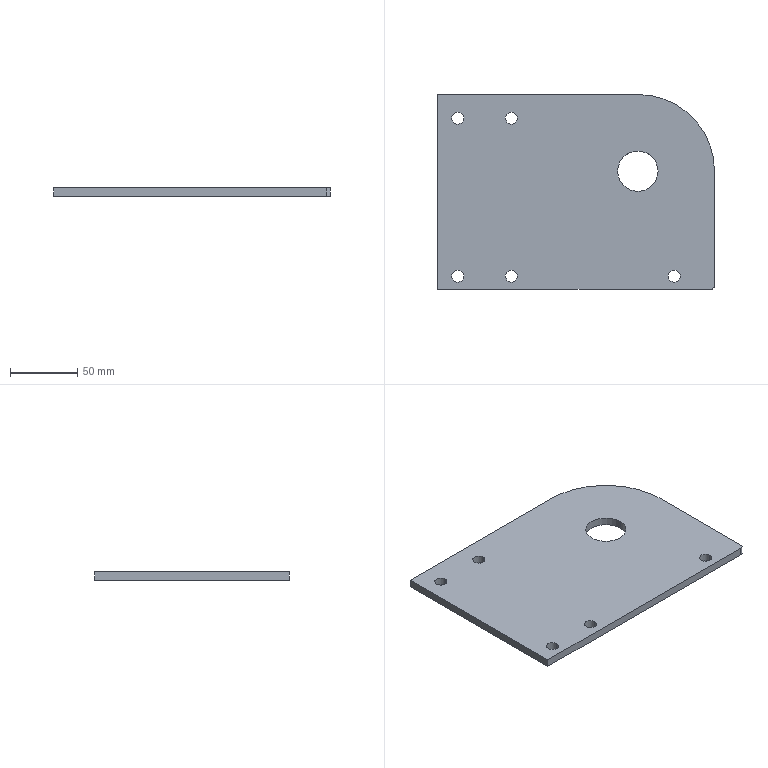Part | SolidWorks | features ICE 6, Fillet 5, HoleWzd 2, CirPattern 1, Extrusion 1 | 1 solid | 20 faces | box 206 x 145 x 6 mm | volume 168875 mm3 | cylinder 14 | plane 6 | commonest cylinder face diameters 9 x10 30 x2 6 x1 114 x1
STEP:
#1=CARTESIAN_POINT('',(68.5,-62.5,0.));
#2=VERTEX_POINT('',#1);
#3=CARTESIAN_POINT('',(77.5,-62.5,0.));
#4=VERTEX_POINT('',#3);
#5=CARTESIAN_POINT('',(73.,-62.5,0.));
#6=DIRECTION('',(0.,0.,1.));
#7=DIRECTION('',(1.,0.,0.));
#8=AXIS2_PLACEMENT_3D('',#5,#6,#7);
#9=CIRCLE('',#8,4.5);
#10=EDGE_CURVE('',#2,#4,#9,.T.);
#11=ORIENTED_EDGE('',*,*,#10,.F.);
#12=CARTESIAN_POINT('',(68.5,-62.5,6.));
#13=VERTEX_POINT('',#12);
#14=CARTESIAN_POINT('',(68.5,-62.5,0.));
#15=DIRECTION('',(0.,0.,1.));
#16=VECTOR('',#15,1000.);
#17=LINE('',#14,#16);
#18=EDGE_CURVE('',#2,#13,#17,.T.);
#19=ORIENTED_EDGE('',*,*,#18,.T.);
#20=CARTESIAN_POINT('',(77.5,-62.5,6.));
#21=VERTEX_POINT('',#20);
#22=CARTESIAN_POINT('',(73.,-62.5,6.));
#23=DIRECTION('',(0.,0.,1.));
#24=DIRECTION('',(1.,0.,0.));
#25=AXIS2_PLACEMENT_3D('',#22,#23,#24);
#26=CIRCLE('',#25,4.5);
#27=EDGE_CURVE('',#13,#21,#26,.T.);
#28=ORIENTED_EDGE('',*,*,#27,.T.);
#29=CARTESIAN_POINT('',(77.5,-62.5,0.));
#30=DIRECTION('',(0.,0.,1.));
#31=VECTOR('',#30,1000.);
#32=LINE('',#29,#31);
#33=EDGE_CURVE('',#4,#21,#32,.T.);
#34=ORIENTED_EDGE('',*,*,#33,.F.);
#35=EDGE_LOOP('',(#11,#19,#28,#34));
#36=FACE_OUTER_BOUND('',#35,.T.);
#37=CARTESIAN_POINT('',(73.,-62.5,0.));
#38=DIRECTION('',(0.,0.,1.));
#39=DIRECTION('',(1.,0.,0.));
#40=AXIS2_PLACEMENT_3D('',#37,#38,#39);
#41=CYLINDRICAL_SURFACE('',#40,4.5);
#42=ADVANCED_FACE('',(#36),#41,.F.);
#43=CARTESIAN_POINT('',(31.,15.5,0.));
#44=VERTEX_POINT('',#43);
#45=CARTESIAN_POINT('',(61.,15.5,0.));
#46=VERTEX_POINT('',#45);
#47=CARTESIAN_POINT('',(46.,15.5,0.));
#48=DIRECTION('',(0.,0.,1.));
#49=DIRECTION('',(1.,0.,0.));
#50=AXIS2_PLACEMENT_3D('',#47,#48,#49);
#51=CIRCLE('',#50,15.);
#52=EDGE_CURVE('',#44,#46,#51,.T.);
#53=ORIENTED_EDGE('',*,*,#52,.F.);
#54=CARTESIAN_POINT('',(31.,15.5,6.));
#55=VERTEX_POINT('',#54);
#56=CARTESIAN_POINT('',(31.,15.5,0.));
#57=DIRECTION('',(0.,0.,1.));
#58=VECTOR('',#57,1000.);
#59=LINE('',#56,#58);
#60=EDGE_CURVE('',#44,#55,#59,.T.);
#61=ORIENTED_EDGE('',*,*,#60,.T.);
#62=CARTESIAN_POINT('',(61.,15.5,6.));
#63=VERTEX_POINT('',#62);
#64=CARTESIAN_POINT('',(46.,15.5,6.));
#65=DIRECTION('',(0.,0.,1.));
#66=DIRECTION('',(1.,0.,0.));
#67=AXIS2_PLACEMENT_3D('',#64,#65,#66);
#68=CIRCLE('',#67,15.);
#69=EDGE_CURVE('',#55,#63,#68,.T.);
#70=ORIENTED_EDGE('',*,*,#69,.T.);
#71=CARTESIAN_POINT('',(61.,15.5,0.));
#72=DIRECTION('',(0.,0.,1.));
#73=VECTOR('',#72,1000.);
#74=LINE('',#71,#73);
#75=EDGE_CURVE('',#46,#63,#74,.T.);
#76=ORIENTED_EDGE('',*,*,#75,.F.);
#77=EDGE_LOOP('',(#53,#61,#70,#76));
#78=FACE_OUTER_BOUND('',#77,.T.);
#79=CARTESIAN_POINT('',(46.,15.5,0.));
#80=DIRECTION('',(0.,0.,1.));
#81=DIRECTION('',(1.,0.,0.));
#82=AXIS2_PLACEMENT_3D('',#79,#80,#81);
#83=CYLINDRICAL_SURFACE('',#82,15.);
#84=ADVANCED_FACE('',(#78),#83,.F.);
#85=CARTESIAN_POINT('',(-52.5,-62.5,0.));
#86=VERTEX_POINT('',#85);
#87=CARTESIAN_POINT('',(-43.5,-62.5,0.));
#88=VERTEX_POINT('',#87);
#89=CARTESIAN_POINT('',(-48.,-62.5,0.));
#90=DIRECTION('',(0.,0.,1.));
#91=DIRECTION('',(1.,0.,0.));
#92=AXIS2_PLACEMENT_3D('',#89,#90,#91);
#93=CIRCLE('',#92,4.5);
#94=EDGE_CURVE('',#86,#88,#93,.T.);
#95=ORIENTED_EDGE('',*,*,#94,.F.);
#96=CARTESIAN_POINT('',(-52.5,-62.5,6.));
#97=VERTEX_POINT('',#96);
#98=CARTESIAN_POINT('',(-52.5,-62.5,0.));
#99=DIRECTION('',(0.,0.,1.));
#100=VECTOR('',#99,1000.);
#101=LINE('',#98,#100);
#102=EDGE_CURVE('',#86,#97,#101,.T.);
#103=ORIENTED_EDGE('',*,*,#102,.T.);
#104=CARTESIAN_POINT('',(-43.5,-62.5,6.));
#105=VERTEX_POINT('',#104);
#106=CARTESIAN_POINT('',(-48.,-62.5,6.));
#107=DIRECTION('',(0.,0.,1.));
#108=DIRECTION('',(1.,0.,0.));
#109=AXIS2_PLACEMENT_3D('',#106,#107,#108);
#110=CIRCLE('',#109,4.5);
#111=EDGE_CURVE('',#97,#105,#110,.T.);
#112=ORIENTED_EDGE('',*,*,#111,.T.);
#113=CARTESIAN_POINT('',(-43.5,-62.5,0.));
#114=DIRECTION('',(0.,0.,1.));
#115=VECTOR('',#114,1000.);
#116=LINE('',#113,#115);
#117=EDGE_CURVE('',#88,#105,#116,.T.);
#118=ORIENTED_EDGE('',*,*,#117,.F.);
#119=EDGE_LOOP('',(#95,#103,#112,#118));
#120=FACE_OUTER_BOUND('',#119,.T.);
#121=CARTESIAN_POINT('',(-48.,-62.5,0.));
#122=DIRECTION('',(0.,0.,1.));
#123=DIRECTION('',(1.,0.,0.));
#124=AXIS2_PLACEMENT_3D('',#121,#122,#123);
#125=CYLINDRICAL_SURFACE('',#124,4.5);
#126=ADVANCED_FACE('',(#120),#125,.F.);
#127=CARTESIAN_POINT('',(-92.5,-62.5,0.));
#128=VERTEX_POINT('',#127);
#129=CARTESIAN_POINT('',(-83.5,-62.5,0.));
#130=VERTEX_POINT('',#129);
#131=CARTESIAN_POINT('',(-88.,-62.5,0.));
#132=DIRECTION('',(0.,0.,1.));
#133=DIRECTION('',(1.,0.,0.));
#134=AXIS2_PLACEMENT_3D('',#131,#132,#133);
#135=CIRCLE('',#134,4.5);
#136=EDGE_CURVE('',#128,#130,#135,.T.);
#137=ORIENTED_EDGE('',*,*,#136,.F.);
#138=CARTESIAN_POINT('',(-92.5,-62.5,6.));
#139=VERTEX_POINT('',#138);
#140=CARTESIAN_POINT('',(-92.5,-62.5,0.));
#141=DIRECTION('',(0.,0.,1.));
#142=VECTOR('',#141,1000.);
#143=LINE('',#140,#142);
#144=EDGE_CURVE('',#128,#139,#143,.T.);
#145=ORIENTED_EDGE('',*,*,#144,.T.);
#146=CARTESIAN_POINT('',(-83.5,-62.5,6.));
#147=VERTEX_POINT('',#146);
#148=CARTESIAN_POINT('',(-88.,-62.5,6.));
#149=DIRECTION('',(0.,0.,1.));
#150=DIRECTION('',(1.,0.,0.));
#151=AXIS2_PLACEMENT_3D('',#148,#149,#150);
#152=CIRCLE('',#151,4.5);
#153=EDGE_CURVE('',#139,#147,#152,.T.);
#154=ORIENTED_EDGE('',*,*,#153,.T.);
#155=CARTESIAN_POINT('',(-83.5,-62.5,0.));
#156=DIRECTION('',(0.,0.,1.));
#157=VECTOR('',#156,1000.);
#158=LINE('',#155,#157);
#159=EDGE_CURVE('',#130,#147,#158,.T.);
#160=ORIENTED_EDGE('',*,*,#159,.F.);
#161=EDGE_LOOP('',(#137,#145,#154,#160));
#162=FACE_OUTER_BOUND('',#161,.T.);
#163=CARTESIAN_POINT('',(-88.,-62.5,0.));
#164=DIRECTION('',(0.,0.,1.));
#165=DIRECTION('',(1.,0.,0.));
#166=AXIS2_PLACEMENT_3D('',#163,#164,#165);
#167=CYLINDRICAL_SURFACE('',#166,4.5);
#168=ADVANCED_FACE('',(#162),#167,.F.);
#169=CARTESIAN_POINT('',(-52.5,55.,0.));
#170=VERTEX_POINT('',#169);
#171=CARTESIAN_POINT('',(-43.5,55.,0.));
#172=VERTEX_POINT('',#171);
#173=CARTESIAN_POINT('',(-48.,55.,0.));
#174=DIRECTION('',(0.,0.,1.));
#175=DIRECTION('',(1.,0.,0.));
#176=AXIS2_PLACEMENT_3D('',#173,#174,#175);
#177=CIRCLE('',#176,4.5);
#178=EDGE_CURVE('',#170,#172,#177,.T.);
#179=ORIENTED_EDGE('',*,*,#178,.F.);
#180=CARTESIAN_POINT('',(-52.5,55.,6.));
#181=VERTEX_POINT('',#180);
#182=CARTESIAN_POINT('',(-52.5,55.,0.));
#183=DIRECTION('',(0.,0.,1.));
#184=VECTOR('',#183,1000.);
#185=LINE('',#182,#184);
#186=EDGE_CURVE('',#170,#181,#185,.T.);
#187=ORIENTED_EDGE('',*,*,#186,.T.);
#188=CARTESIAN_POINT('',(-43.5,55.,6.));
#189=VERTEX_POINT('',#188);
#190=CARTESIAN_POINT('',(-48.,55.,6.));
#191=DIRECTION('',(0.,0.,1.));
#192=DIRECTION('',(1.,0.,0.));
#193=AXIS2_PLACEMENT_3D('',#190,#191,#192);
#194=CIRCLE('',#193,4.5);
#195=EDGE_CURVE('',#181,#189,#194,.T.);
#196=ORIENTED_EDGE('',*,*,#195,.T.);
#197=CARTESIAN_POINT('',(-43.5,55.,0.));
#198=DIRECTION('',(0.,0.,1.));
#199=VECTOR('',#198,1000.);
#200=LINE('',#197,#199);
#201=EDGE_CURVE('',#172,#189,#200,.T.);
#202=ORIENTED_EDGE('',*,*,#201,.F.);
#203=EDGE_LOOP('',(#179,#187,#196,#202));
#204=FACE_OUTER_BOUND('',#203,.T.);
#205=CARTESIAN_POINT('',(-48.,55.,0.));
#206=DIRECTION('',(0.,0.,1.));
#207=DIRECTION('',(1.,0.,0.));
#208=AXIS2_PLACEMENT_3D('',#205,#206,#207);
#209=CYLINDRICAL_SURFACE('',#208,4.5);
#210=ADVANCED_FACE('',(#204),#209,.F.);
#211=CARTESIAN_POINT('',(-92.5,55.,0.));
#212=VERTEX_POINT('',#211);
#213=CARTESIAN_POINT('',(-83.5,55.,0.));
#214=VERTEX_POINT('',#213);
#215=CARTESIAN_POINT('',(-88.,55.,0.));
#216=DIRECTION('',(0.,0.,1.));
#217=DIRECTION('',(1.,0.,0.));
#218=AXIS2_PLACEMENT_3D('',#215,#216,#217);
#219=CIRCLE('',#218,4.5);
#220=EDGE_CURVE('',#212,#214,#219,.T.);
#221=ORIENTED_EDGE('',*,*,#220,.F.);
#222=CARTESIAN_POINT('',(-92.5,55.,6.));
#223=VERTEX_POINT('',#222);
#224=CARTESIAN_POINT('',(-92.5,55.,0.));
#225=DIRECTION('',(0.,0.,1.));
#226=VECTOR('',#225,1000.);
#227=LINE('',#224,#226);
#228=EDGE_CURVE('',#212,#223,#227,.T.);
#229=ORIENTED_EDGE('',*,*,#228,.T.);
#230=CARTESIAN_POINT('',(-83.5,55.,6.));
#231=VERTEX_POINT('',#230);
#232=CARTESIAN_POINT('',(-88.,55.,6.));
#233=DIRECTION('',(0.,0.,1.));
#234=DIRECTION('',(1.,0.,0.));
#235=AXIS2_PLACEMENT_3D('',#232,#233,#234);
#236=CIRCLE('',#235,4.5);
#237=EDGE_CURVE('',#223,#231,#236,.T.);
#238=ORIENTED_EDGE('',*,*,#237,.T.);
#239=CARTESIAN_POINT('',(-83.5,55.,0.));
#240=DIRECTION('',(0.,0.,1.));
#241=VECTOR('',#240,1000.);
#242=LINE('',#239,#241);
#243=EDGE_CURVE('',#214,#231,#242,.T.);
#244=ORIENTED_EDGE('',*,*,#243,.F.);
#245=EDGE_LOOP('',(#221,#229,#238,#244));
#246=FACE_OUTER_BOUND('',#245,.T.);
#247=CARTESIAN_POINT('',(-88.,55.,0.));
#248=DIRECTION('',(0.,0.,1.));
#249=DIRECTION('',(1.,0.,0.));
#250=AXIS2_PLACEMENT_3D('',#247,#248,#249);
#251=CYLINDRICAL_SURFACE('',#250,4.5);
#252=ADVANCED_FACE('',(#246),#251,.F.);
#253=CARTESIAN_POINT('',(-103.,72.5,0.));
#254=VERTEX_POINT('',#253);
#255=CARTESIAN_POINT('',(-103.,-72.5,0.));
#256=VERTEX_POINT('',#255);
#257=CARTESIAN_POINT('',(-103.,72.5,0.));
#258=DIRECTION('',(0.,-1.,0.));
#259=VECTOR('',#258,1000.);
#260=LINE('',#257,#259);
#261=EDGE_CURVE('',#254,#256,#260,.T.);
#262=ORIENTED_EDGE('',*,*,#261,.T.);
#263=CARTESIAN_POINT('',(-103.,-72.5,6.));
#264=VERTEX_POINT('',#263);
#265=CARTESIAN_POINT('',(-103.,-72.5,6.));
#266=DIRECTION('',(0.,0.,-1.));
#267=VECTOR('',#266,1000.);
#268=LINE('',#265,#267);
#269=EDGE_CURVE('',#264,#256,#268,.T.);
#270=ORIENTED_EDGE('',*,*,#269,.F.);
#271=CARTESIAN_POINT('',(-103.,72.5,6.));
#272=VERTEX_POINT('',#271);
#273=CARTESIAN_POINT('',(-103.,72.5,6.));
#274=DIRECTION('',(0.,-1.,0.));
#275=VECTOR('',#274,1000.);
#276=LINE('',#273,#275);
#277=EDGE_CURVE('',#272,#264,#276,.T.);
#278=ORIENTED_EDGE('',*,*,#277,.F.);
#279=CARTESIAN_POINT('',(-103.,72.5,6.));
#280=DIRECTION('',(0.,0.,-1.));
#281=VECTOR('',#280,1000.);
#282=LINE('',#279,#281);
#283=EDGE_CURVE('',#272,#254,#282,.T.);
#284=ORIENTED_EDGE('',*,*,#283,.T.);
#285=EDGE_LOOP('',(#262,#270,#278,#284));
#286=FACE_OUTER_BOUND('',#285,.T.);
#287=CARTESIAN_POINT('',(-103.,72.5,6.));
#288=DIRECTION('',(1.,0.,0.));
#289=DIRECTION('',(0.,0.,-1.));
#290=AXIS2_PLACEMENT_3D('',#287,#288,#289);
#291=PLANE('',#290);
#292=ADVANCED_FACE('',(#286),#291,.F.);
#293=CARTESIAN_POINT('',(100.,-72.5,0.));
#294=VERTEX_POINT('',#293);
#295=CARTESIAN_POINT('',(-103.,-72.5,0.));
#296=DIRECTION('',(1.,0.,0.));
#297=VECTOR('',#296,1000.);
#298=LINE('',#295,#297);
#299=EDGE_CURVE('',#256,#294,#298,.T.);
#300=ORIENTED_EDGE('',*,*,#299,.T.);
#301=CARTESIAN_POINT('',(100.,-72.5,6.));
#302=VERTEX_POINT('',#301);
#303=CARTESIAN_POINT('',(100.,-72.5,6.));
#304=DIRECTION('',(0.,0.,1.));
#305=VECTOR('',#304,1000.);
#306=LINE('',#303,#305);
#307=EDGE_CURVE('',#294,#302,#306,.T.);
#308=ORIENTED_EDGE('',*,*,#307,.T.);
#309=CARTESIAN_POINT('',(-103.,-72.5,6.));
#310=DIRECTION('',(1.,0.,0.));
#311=VECTOR('',#310,1000.);
#312=LINE('',#309,#311);
#313=EDGE_CURVE('',#264,#302,#312,.T.);
#314=ORIENTED_EDGE('',*,*,#313,.F.);
#315=ORIENTED_EDGE('',*,*,#269,.T.);
#316=EDGE_LOOP('',(#300,#308,#314,#315));
#317=FACE_OUTER_BOUND('',#316,.T.);
#318=CARTESIAN_POINT('',(-103.,-72.5,6.));
#319=DIRECTION('',(0.,1.,0.));
#320=DIRECTION('',(0.,0.,1.));
#321=AXIS2_PLACEMENT_3D('',#318,#319,#320);
#322=PLANE('',#321);
#323=ADVANCED_FACE('',(#317),#322,.F.);
#324=CARTESIAN_POINT('',(103.,-69.5,6.));
#325=VERTEX_POINT('',#324);
#326=CARTESIAN_POINT('',(103.,15.5,6.));
#327=VERTEX_POINT('',#326);
#328=CARTESIAN_POINT('',(103.,72.5,6.));
#329=DIRECTION('',(0.,1.,0.));
#330=VECTOR('',#329,1000.);
#331=LINE('',#328,#330);
#332=EDGE_CURVE('',#325,#327,#331,.T.);
#333=ORIENTED_EDGE('',*,*,#332,.F.);
#334=CARTESIAN_POINT('',(103.,-69.5,0.));
#335=VERTEX_POINT('',#334);
#336=CARTESIAN_POINT('',(103.,-69.5,6.));
#337=DIRECTION('',(0.,0.,-1.));
#338=VECTOR('',#337,1000.);
#339=LINE('',#336,#338);
#340=EDGE_CURVE('',#325,#335,#339,.T.);
#341=ORIENTED_EDGE('',*,*,#340,.T.);
#342=CARTESIAN_POINT('',(103.,15.5,0.));
#343=VERTEX_POINT('',#342);
#344=CARTESIAN_POINT('',(103.,72.5,0.));
#345=DIRECTION('',(0.,1.,0.));
#346=VECTOR('',#345,1000.);
#347=LINE('',#344,#346);
#348=EDGE_CURVE('',#335,#343,#347,.T.);
#349=ORIENTED_EDGE('',*,*,#348,.T.);
#350=CARTESIAN_POINT('',(103.,15.5,6.));
#351=DIRECTION('',(0.,0.,1.));
#352=VECTOR('',#351,1000.);
#353=LINE('',#350,#352);
#354=EDGE_CURVE('',#343,#327,#353,.T.);
#355=ORIENTED_EDGE('',*,*,#354,.T.);
#356=EDGE_LOOP('',(#333,#341,#349,#355));
#357=FACE_OUTER_BOUND('',#356,.T.);
#358=CARTESIAN_POINT('',(103.,72.5,6.));
#359=DIRECTION('',(-1.,0.,0.));
#360=DIRECTION('',(0.,0.,1.));
#361=AXIS2_PLACEMENT_3D('',#358,#359,#360);
#362=PLANE('',#361);
#363=ADVANCED_FACE('',(#357),#362,.F.);
#364=CARTESIAN_POINT('',(46.,72.5,6.));
#365=VERTEX_POINT('',#364);
#366=CARTESIAN_POINT('',(-103.,72.5,6.));
#367=DIRECTION('',(-1.,0.,0.));
#368=VECTOR('',#367,1000.);
#369=LINE('',#366,#368);
#370=EDGE_CURVE('',#365,#272,#369,.T.);
#371=ORIENTED_EDGE('',*,*,#370,.F.);
#372=CARTESIAN_POINT('',(46.,72.5,0.));
#373=VERTEX_POINT('',#372);
#374=CARTESIAN_POINT('',(46.,72.5,6.));
#375=DIRECTION('',(0.,0.,-1.));
#376=VECTOR('',#375,1000.);
#377=LINE('',#374,#376);
#378=EDGE_CURVE('',#365,#373,#377,.T.);
#379=ORIENTED_EDGE('',*,*,#378,.T.);
#380=CARTESIAN_POINT('',(-103.,72.5,0.));
#381=DIRECTION('',(-1.,0.,0.));
#382=VECTOR('',#381,1000.);
#383=LINE('',#380,#382);
#384=EDGE_CURVE('',#373,#254,#383,.T.);
#385=ORIENTED_EDGE('',*,*,#384,.T.);
#386=ORIENTED_EDGE('',*,*,#283,.F.);
#387=EDGE_LOOP('',(#371,#379,#385,#386));
#388=FACE_OUTER_BOUND('',#387,.T.);
#389=CARTESIAN_POINT('',(-103.,72.5,6.));
#390=DIRECTION('',(0.,-1.,0.));
#391=DIRECTION('',(0.,0.,-1.));
#392=AXIS2_PLACEMENT_3D('',#389,#390,#391);
#393=PLANE('',#392);
#394=ADVANCED_FACE('',(#388),#393,.F.);
#395=CARTESIAN_POINT('',(73.,-62.5,6.));
#396=DIRECTION('',(0.,0.,1.));
#397=DIRECTION('',(1.,0.,0.));
#398=AXIS2_PLACEMENT_3D('',#395,#396,#397);
#399=CIRCLE('',#398,4.5);
#400=EDGE_CURVE('',#21,#13,#399,.T.);
#401=ORIENTED_EDGE('',*,*,#400,.F.);
#402=ORIENTED_EDGE('',*,*,#27,.F.);
#403=EDGE_LOOP('',(#401,#402));
#404=FACE_BOUND('',#403,.T.);
#405=CARTESIAN_POINT('',(46.,15.5,6.));
#406=DIRECTION('',(0.,0.,1.));
#407=DIRECTION('',(1.,0.,0.));
#408=AXIS2_PLACEMENT_3D('',#405,#406,#407);
#409=CIRCLE('',#408,15.);
#410=EDGE_CURVE('',#63,#55,#409,.T.);
#411=ORIENTED_EDGE('',*,*,#410,.F.);
#412=ORIENTED_EDGE('',*,*,#69,.F.);
#413=EDGE_LOOP('',(#411,#412));
#414=FACE_BOUND('',#413,.T.);
#415=CARTESIAN_POINT('',(-48.,-62.5,6.));
#416=DIRECTION('',(0.,0.,1.));
#417=DIRECTION('',(1.,0.,0.));
#418=AXIS2_PLACEMENT_3D('',#415,#416,#417);
#419=CIRCLE('',#418,4.5);
#420=EDGE_CURVE('',#105,#97,#419,.T.);
#421=ORIENTED_EDGE('',*,*,#420,.F.);
#422=ORIENTED_EDGE('',*,*,#111,.F.);
#423=EDGE_LOOP('',(#421,#422));
#424=FACE_BOUND('',#423,.T.);
#425=CARTESIAN_POINT('',(-88.,-62.5,6.));
#426=DIRECTION('',(0.,0.,1.));
#427=DIRECTION('',(1.,0.,0.));
#428=AXIS2_PLACEMENT_3D('',#425,#426,#427);
#429=CIRCLE('',#428,4.5);
#430=EDGE_CURVE('',#147,#139,#429,.T.);
#431=ORIENTED_EDGE('',*,*,#430,.F.);
#432=ORIENTED_EDGE('',*,*,#153,.F.);
#433=EDGE_LOOP('',(#431,#432));
#434=FACE_BOUND('',#433,.T.);
#435=CARTESIAN_POINT('',(-48.,55.,6.));
#436=DIRECTION('',(0.,0.,1.));
#437=DIRECTION('',(1.,0.,0.));
#438=AXIS2_PLACEMENT_3D('',#435,#436,#437);
#439=CIRCLE('',#438,4.5);
#440=EDGE_CURVE('',#189,#181,#439,.T.);
#441=ORIENTED_EDGE('',*,*,#440,.F.);
#442=ORIENTED_EDGE('',*,*,#195,.F.);
#443=EDGE_LOOP('',(#441,#442));
#444=FACE_BOUND('',#443,.T.);
#445=CARTESIAN_POINT('',(-88.,55.,6.));
#446=DIRECTION('',(0.,0.,1.));
#447=DIRECTION('',(1.,0.,0.));
#448=AXIS2_PLACEMENT_3D('',#445,#446,#447);
#449=CIRCLE('',#448,4.5);
#450=EDGE_CURVE('',#231,#223,#449,.T.);
#451=ORIENTED_EDGE('',*,*,#450,.F.);
#452=ORIENTED_EDGE('',*,*,#237,.F.);
#453=EDGE_LOOP('',(#451,#452));
#454=FACE_BOUND('',#453,.T.);
#455=ORIENTED_EDGE('',*,*,#313,.T.);
#456=CARTESIAN_POINT('',(100.,-69.5,6.));
#457=DIRECTION('',(0.,0.,1.));
#458=DIRECTION('',(1.,0.,0.));
#459=AXIS2_PLACEMENT_3D('',#456,#457,#458);
#460=CIRCLE('',#459,3.);
#461=EDGE_CURVE('',#302,#325,#460,.T.);
#462=ORIENTED_EDGE('',*,*,#461,.T.);
#463=ORIENTED_EDGE('',*,*,#332,.T.);
#464=CARTESIAN_POINT('',(46.,15.5,6.));
#465=DIRECTION('',(0.,0.,1.));
#466=DIRECTION('',(1.,0.,0.));
#467=AXIS2_PLACEMENT_3D('',#464,#465,#466);
#468=CIRCLE('',#467,57.);
#469=EDGE_CURVE('',#327,#365,#468,.T.);
#470=ORIENTED_EDGE('',*,*,#469,.T.);
#471=ORIENTED_EDGE('',*,*,#370,.T.);
#472=ORIENTED_EDGE('',*,*,#277,.T.);
#473=EDGE_LOOP('',(#455,#462,#463,#470,#471,#472));
#474=FACE_OUTER_BOUND('',#473,.T.);
#475=CARTESIAN_POINT('',(0.,0.,6.));
#476=DIRECTION('',(0.,0.,1.));
#477=DIRECTION('',(1.,0.,0.));
#478=AXIS2_PLACEMENT_3D('',#475,#476,#477);
#479=PLANE('',#478);
#480=ADVANCED_FACE('',(#404,#414,#424,#434,#444,#454,#474),#479,.T.);
#481=CARTESIAN_POINT('',(73.,-62.5,0.));
#482=DIRECTION('',(0.,0.,1.));
#483=DIRECTION('',(1.,0.,0.));
#484=AXIS2_PLACEMENT_3D('',#481,#482,#483);
#485=CIRCLE('',#484,4.5);
#486=EDGE_CURVE('',#4,#2,#485,.T.);
#487=ORIENTED_EDGE('',*,*,#486,.T.);
#488=ORIENTED_EDGE('',*,*,#10,.T.);
#489=EDGE_LOOP('',(#487,#488));
#490=FACE_BOUND('',#489,.T.);
#491=CARTESIAN_POINT('',(46.,15.5,0.));
#492=DIRECTION('',(0.,0.,1.));
#493=DIRECTION('',(1.,0.,0.));
#494=AXIS2_PLACEMENT_3D('',#491,#492,#493);
#495=CIRCLE('',#494,15.);
#496=EDGE_CURVE('',#46,#44,#495,.T.);
#497=ORIENTED_EDGE('',*,*,#496,.T.);
#498=ORIENTED_EDGE('',*,*,#52,.T.);
#499=EDGE_LOOP('',(#497,#498));
#500=FACE_BOUND('',#499,.T.);
#501=CARTESIAN_POINT('',(-48.,-62.5,0.));
#502=DIRECTION('',(0.,0.,1.));
#503=DIRECTION('',(1.,0.,0.));
#504=AXIS2_PLACEMENT_3D('',#501,#502,#503);
#505=CIRCLE('',#504,4.5);
#506=EDGE_CURVE('',#88,#86,#505,.T.);
#507=ORIENTED_EDGE('',*,*,#506,.T.);
#508=ORIENTED_EDGE('',*,*,#94,.T.);
#509=EDGE_LOOP('',(#507,#508));
#510=FACE_BOUND('',#509,.T.);
#511=CARTESIAN_POINT('',(-88.,-62.5,0.));
#512=DIRECTION('',(0.,0.,1.));
#513=DIRECTION('',(1.,0.,0.));
#514=AXIS2_PLACEMENT_3D('',#511,#512,#513);
#515=CIRCLE('',#514,4.5);
#516=EDGE_CURVE('',#130,#128,#515,.T.);
#517=ORIENTED_EDGE('',*,*,#516,.T.);
#518=ORIENTED_EDGE('',*,*,#136,.T.);
#519=EDGE_LOOP('',(#517,#518));
#520=FACE_BOUND('',#519,.T.);
#521=CARTESIAN_POINT('',(-48.,55.,0.));
#522=DIRECTION('',(0.,0.,1.));
#523=DIRECTION('',(1.,0.,0.));
#524=AXIS2_PLACEMENT_3D('',#521,#522,#523);
#525=CIRCLE('',#524,4.5);
#526=EDGE_CURVE('',#172,#170,#525,.T.);
#527=ORIENTED_EDGE('',*,*,#526,.T.);
#528=ORIENTED_EDGE('',*,*,#178,.T.);
#529=EDGE_LOOP('',(#527,#528));
#530=FACE_BOUND('',#529,.T.);
#531=CARTESIAN_POINT('',(-88.,55.,0.));
#532=DIRECTION('',(0.,0.,1.));
#533=DIRECTION('',(1.,0.,0.));
#534=AXIS2_PLACEMENT_3D('',#531,#532,#533);
#535=CIRCLE('',#534,4.5);
#536=EDGE_CURVE('',#214,#212,#535,.T.);
#537=ORIENTED_EDGE('',*,*,#536,.T.);
#538=ORIENTED_EDGE('',*,*,#220,.T.);
#539=EDGE_LOOP('',(#537,#538));
#540=FACE_BOUND('',#539,.T.);
#541=ORIENTED_EDGE('',*,*,#348,.F.);
#542=CARTESIAN_POINT('',(100.,-69.5,0.));
#543=DIRECTION('',(0.,0.,-1.));
#544=DIRECTION('',(1.,0.,0.));
#545=AXIS2_PLACEMENT_3D('',#542,#543,#544);
#546=CIRCLE('',#545,3.);
#547=EDGE_CURVE('',#335,#294,#546,.T.);
#548=ORIENTED_EDGE('',*,*,#547,.T.);
#549=ORIENTED_EDGE('',*,*,#299,.F.);
#550=ORIENTED_EDGE('',*,*,#261,.F.);
#551=ORIENTED_EDGE('',*,*,#384,.F.);
#552=CARTESIAN_POINT('',(46.,15.5,0.));
#553=DIRECTION('',(0.,0.,-1.));
#554=DIRECTION('',(1.,0.,0.));
#555=AXIS2_PLACEMENT_3D('',#552,#553,#554);
#556=CIRCLE('',#555,57.);
#557=EDGE_CURVE('',#373,#343,#556,.T.);
#558=ORIENTED_EDGE('',*,*,#557,.T.);
#559=EDGE_LOOP('',(#541,#548,#549,#550,#551,#558));
#560=FACE_OUTER_BOUND('',#559,.T.);
#561=CARTESIAN_POINT('',(0.,0.,0.));
#562=DIRECTION('',(0.,0.,1.));
#563=DIRECTION('',(1.,0.,0.));
#564=AXIS2_PLACEMENT_3D('',#561,#562,#563);
#565=PLANE('',#564);
#566=ADVANCED_FACE('',(#490,#500,#510,#520,#530,#540,#560),#565,.F.);
#567=ORIENTED_EDGE('',*,*,#228,.F.);
#568=ORIENTED_EDGE('',*,*,#536,.F.);
#569=ORIENTED_EDGE('',*,*,#243,.T.);
#570=ORIENTED_EDGE('',*,*,#450,.T.);
#571=EDGE_LOOP('',(#567,#568,#569,#570));
#572=FACE_OUTER_BOUND('',#571,.T.);
#573=CARTESIAN_POINT('',(-88.,55.,0.));
#574=DIRECTION('',(0.,0.,1.));
#575=DIRECTION('',(1.,0.,0.));
#576=AXIS2_PLACEMENT_3D('',#573,#574,#575);
#577=CYLINDRICAL_SURFACE('',#576,4.5);
#578=ADVANCED_FACE('',(#572),#577,.F.);
#579=ORIENTED_EDGE('',*,*,#186,.F.);
#580=ORIENTED_EDGE('',*,*,#526,.F.);
#581=ORIENTED_EDGE('',*,*,#201,.T.);
#582=ORIENTED_EDGE('',*,*,#440,.T.);
#583=EDGE_LOOP('',(#579,#580,#581,#582));
#584=FACE_OUTER_BOUND('',#583,.T.);
#585=CARTESIAN_POINT('',(-48.,55.,0.));
#586=DIRECTION('',(0.,0.,1.));
#587=DIRECTION('',(1.,0.,0.));
#588=AXIS2_PLACEMENT_3D('',#585,#586,#587);
#589=CYLINDRICAL_SURFACE('',#588,4.5);
#590=ADVANCED_FACE('',(#584),#589,.F.);
#591=ORIENTED_EDGE('',*,*,#144,.F.);
#592=ORIENTED_EDGE('',*,*,#516,.F.);
#593=ORIENTED_EDGE('',*,*,#159,.T.);
#594=ORIENTED_EDGE('',*,*,#430,.T.);
#595=EDGE_LOOP('',(#591,#592,#593,#594));
#596=FACE_OUTER_BOUND('',#595,.T.);
#597=CARTESIAN_POINT('',(-88.,-62.5,0.));
#598=DIRECTION('',(0.,0.,1.));
#599=DIRECTION('',(1.,0.,0.));
#600=AXIS2_PLACEMENT_3D('',#597,#598,#599);
#601=CYLINDRICAL_SURFACE('',#600,4.5);
#602=ADVANCED_FACE('',(#596),#601,.F.);
#603=ORIENTED_EDGE('',*,*,#102,.F.);
#604=ORIENTED_EDGE('',*,*,#506,.F.);
#605=ORIENTED_EDGE('',*,*,#117,.T.);
#606=ORIENTED_EDGE('',*,*,#420,.T.);
#607=EDGE_LOOP('',(#603,#604,#605,#606));
#608=FACE_OUTER_BOUND('',#607,.T.);
#609=CARTESIAN_POINT('',(-48.,-62.5,0.));
#610=DIRECTION('',(0.,0.,1.));
#611=DIRECTION('',(1.,0.,0.));
#612=AXIS2_PLACEMENT_3D('',#609,#610,#611);
#613=CYLINDRICAL_SURFACE('',#612,4.5);
#614=ADVANCED_FACE('',(#608),#613,.F.);
#615=ORIENTED_EDGE('',*,*,#60,.F.);
#616=ORIENTED_EDGE('',*,*,#496,.F.);
#617=ORIENTED_EDGE('',*,*,#75,.T.);
#618=ORIENTED_EDGE('',*,*,#410,.T.);
#619=EDGE_LOOP('',(#615,#616,#617,#618));
#620=FACE_OUTER_BOUND('',#619,.T.);
#621=CARTESIAN_POINT('',(46.,15.5,0.));
#622=DIRECTION('',(0.,0.,1.));
#623=DIRECTION('',(1.,0.,0.));
#624=AXIS2_PLACEMENT_3D('',#621,#622,#623);
#625=CYLINDRICAL_SURFACE('',#624,15.);
#626=ADVANCED_FACE('',(#620),#625,.F.);
#627=ORIENTED_EDGE('',*,*,#469,.F.);
#628=ORIENTED_EDGE('',*,*,#354,.F.);
#629=ORIENTED_EDGE('',*,*,#557,.F.);
#630=ORIENTED_EDGE('',*,*,#378,.F.);
#631=EDGE_LOOP('',(#627,#628,#629,#630));
#632=FACE_OUTER_BOUND('',#631,.T.);
#633=CARTESIAN_POINT('',(46.,15.5,6.));
#634=DIRECTION('',(0.,0.,-1.));
#635=DIRECTION('',(-1.,0.,0.));
#636=AXIS2_PLACEMENT_3D('',#633,#634,#635);
#637=CYLINDRICAL_SURFACE('',#636,57.);
#638=ADVANCED_FACE('',(#632),#637,.T.);
#639=ORIENTED_EDGE('',*,*,#18,.F.);
#640=ORIENTED_EDGE('',*,*,#486,.F.);
#641=ORIENTED_EDGE('',*,*,#33,.T.);
#642=ORIENTED_EDGE('',*,*,#400,.T.);
#643=EDGE_LOOP('',(#639,#640,#641,#642));
#644=FACE_OUTER_BOUND('',#643,.T.);
#645=CARTESIAN_POINT('',(73.,-62.5,0.));
#646=DIRECTION('',(0.,0.,1.));
#647=DIRECTION('',(1.,0.,0.));
#648=AXIS2_PLACEMENT_3D('',#645,#646,#647);
#649=CYLINDRICAL_SURFACE('',#648,4.5);
#650=ADVANCED_FACE('',(#644),#649,.F.);
#651=ORIENTED_EDGE('',*,*,#461,.F.);
#652=ORIENTED_EDGE('',*,*,#307,.F.);
#653=ORIENTED_EDGE('',*,*,#547,.F.);
#654=ORIENTED_EDGE('',*,*,#340,.F.);
#655=EDGE_LOOP('',(#651,#652,#653,#654));
#656=FACE_OUTER_BOUND('',#655,.T.);
#657=CARTESIAN_POINT('',(100.,-69.5,6.));
#658=DIRECTION('',(0.,0.,-1.));
#659=DIRECTION('',(-1.,0.,0.));
#660=AXIS2_PLACEMENT_3D('',#657,#658,#659);
#661=CYLINDRICAL_SURFACE('',#660,3.);
#662=ADVANCED_FACE('',(#656),#661,.T.);
#663=CLOSED_SHELL('',(#42,#84,#126,#168,#210,#252,#292,#323,#363,#394,#480,#566,#578,#590,#602,#614,#626,#638,#650,#662));
#664=MANIFOLD_SOLID_BREP('',#663);
#665=CARTESIAN_POINT('',(0.,0.,0.));
#666=DIRECTION('',(0.,0.,1.));
#667=DIRECTION('',(1.,0.,0.));
#668=AXIS2_PLACEMENT_3D('',#665,#666,#667);
#669=(LENGTH_UNIT()NAMED_UNIT(*)SI_UNIT(.MILLI.,.METRE.));
#670=UNCERTAINTY_MEASURE_WITH_UNIT(LENGTH_MEASURE(0.00001),#669,'','');
#671=(NAMED_UNIT(*)PLANE_ANGLE_UNIT()SI_UNIT($,.RADIAN.));
#672=(NAMED_UNIT(*)SI_UNIT($,.STERADIAN.)SOLID_ANGLE_UNIT());
#673=(GEOMETRIC_REPRESENTATION_CONTEXT(3)GLOBAL_UNCERTAINTY_ASSIGNED_CONTEXT((#670))GLOBAL_UNIT_ASSIGNED_CONTEXT((#669,#671,#672))REPRESENTATION_CONTEXT('',''));
#674=ADVANCED_BREP_SHAPE_REPRESENTATION('',(#664,#668),#673);